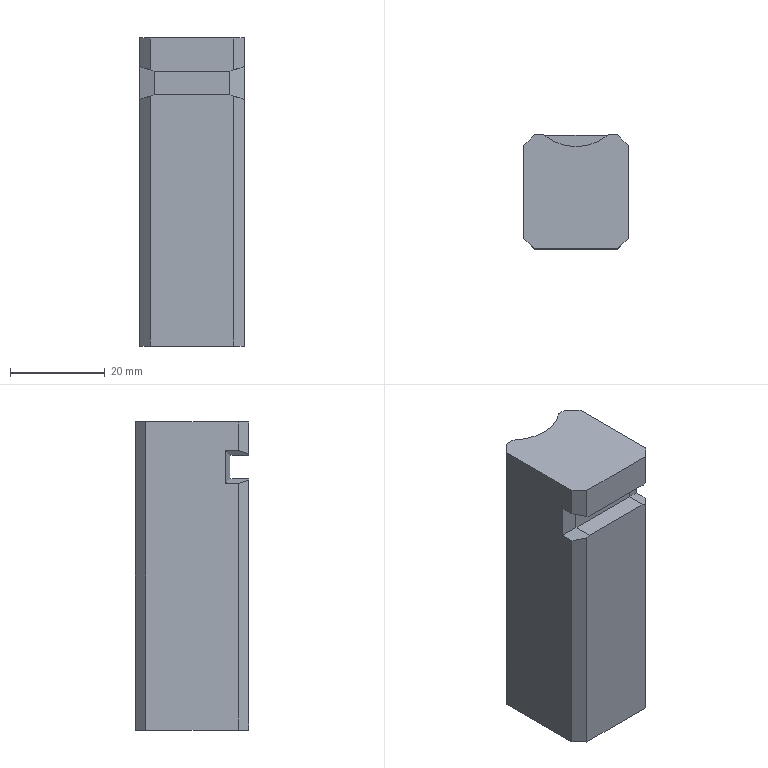Part | NX | features DIE-5 2 | 1 solid | 26 faces | box 22 x 24 x 65 mm | volume 30873 mm3 | plane 24 | cylinder 2 | commonest cylinder face diameters 18.003 x1 21 x1
STEP:
#1=CARTESIAN_POINT('',(2498.895,-772.622,823.716));
#2=VERTEX_POINT('',#1);
#3=CARTESIAN_POINT('',(2485.293,-772.622,823.716));
#4=VERTEX_POINT('',#3);
#5=CARTESIAN_POINT('',(2492.094,-764.622,823.716));
#6=DIRECTION('',(0.,0.,1.));
#7=DIRECTION('',(-1.,0.,0.));
#8=AXIS2_PLACEMENT_3D('',#5,#6,#7);
#9=CIRCLE('',#8,10.5);
#10=EDGE_CURVE('',#2,#4,#9,.F.);
#11=ORIENTED_EDGE('',*,*,#10,.F.);
#12=CARTESIAN_POINT('',(2500.894,-772.622,823.716));
#13=DIRECTION('',(1.,0.,0.));
#14=VECTOR('',#13,1000.);
#15=LINE('',#12,#14);
#16=EDGE_CURVE('',#4,#2,#15,.T.);
#17=ORIENTED_EDGE('',*,*,#16,.F.);
#18=EDGE_LOOP('',(#11,#17));
#19=FACE_BOUND('',#18,.T.);
#20=CARTESIAN_POINT('',(2325.094,-923.422,823.716));
#21=DIRECTION('',(0.,0.,-1.));
#22=DIRECTION('',(-1.,0.,0.));
#23=AXIS2_PLACEMENT_3D('',#20,#21,#22);
#24=PLANE('',#23);
#25=ADVANCED_FACE('',(#19),#24,.F.);
#26=CARTESIAN_POINT('',(2483.294,-772.622,805.716));
#27=VERTEX_POINT('',#26);
#28=CARTESIAN_POINT('',(2483.294,-772.622,870.716));
#29=VERTEX_POINT('',#28);
#30=CARTESIAN_POINT('',(2483.294,-772.622,776.516));
#31=DIRECTION('',(0.,0.,1.));
#32=VECTOR('',#31,1000.);
#33=LINE('',#30,#32);
#34=EDGE_CURVE('',#27,#29,#33,.T.);
#35=ORIENTED_EDGE('',*,*,#34,.T.);
#36=CARTESIAN_POINT('',(2485.293,-772.622,870.716));
#37=VERTEX_POINT('',#36);
#38=CARTESIAN_POINT('',(2492.094,-772.622,870.716));
#39=DIRECTION('',(-1.,0.,0.));
#40=VECTOR('',#39,1000.);
#41=LINE('',#38,#40);
#42=EDGE_CURVE('',#37,#29,#41,.T.);
#43=ORIENTED_EDGE('',*,*,#42,.F.);
#44=CARTESIAN_POINT('',(2485.293,-772.622,839.716));
#45=DIRECTION('',(0.,0.,-1.));
#46=VECTOR('',#45,1000.);
#47=LINE('',#44,#46);
#48=EDGE_CURVE('',#37,#4,#47,.T.);
#49=ORIENTED_EDGE('',*,*,#48,.T.);
#50=ORIENTED_EDGE('',*,*,#16,.T.);
#51=CARTESIAN_POINT('',(2498.895,-772.622,870.716));
#52=VERTEX_POINT('',#51);
#53=CARTESIAN_POINT('',(2498.895,-772.622,839.716));
#54=DIRECTION('',(0.,0.,1.));
#55=VECTOR('',#54,1000.);
#56=LINE('',#53,#55);
#57=EDGE_CURVE('',#2,#52,#56,.T.);
#58=ORIENTED_EDGE('',*,*,#57,.T.);
#59=CARTESIAN_POINT('',(2500.894,-772.622,870.716));
#60=VERTEX_POINT('',#59);
#61=CARTESIAN_POINT('',(2492.094,-772.622,870.716));
#62=DIRECTION('',(-1.,0.,0.));
#63=VECTOR('',#62,1000.);
#64=LINE('',#61,#63);
#65=EDGE_CURVE('',#60,#52,#64,.T.);
#66=ORIENTED_EDGE('',*,*,#65,.F.);
#67=CARTESIAN_POINT('',(2500.894,-772.622,805.716));
#68=VERTEX_POINT('',#67);
#69=CARTESIAN_POINT('',(2500.894,-772.622,776.516));
#70=DIRECTION('',(0.,0.,1.));
#71=VECTOR('',#70,1000.);
#72=LINE('',#69,#71);
#73=EDGE_CURVE('',#68,#60,#72,.T.);
#74=ORIENTED_EDGE('',*,*,#73,.F.);
#75=CARTESIAN_POINT('',(2500.894,-772.622,805.716));
#76=DIRECTION('',(-1.,0.,0.));
#77=VECTOR('',#76,1000.);
#78=LINE('',#75,#77);
#79=EDGE_CURVE('',#68,#27,#78,.T.);
#80=ORIENTED_EDGE('',*,*,#79,.T.);
#81=EDGE_LOOP('',(#35,#43,#49,#50,#58,#66,#74,#80));
#82=FACE_BOUND('',#81,.T.);
#83=CARTESIAN_POINT('',(2500.894,-772.622,776.516));
#84=DIRECTION('',(0.,1.,0.));
#85=DIRECTION('',(1.,0.,0.));
#86=AXIS2_PLACEMENT_3D('',#83,#84,#85);
#87=PLANE('',#86);
#88=ADVANCED_FACE('',(#82),#87,.T.);
#89=CARTESIAN_POINT('',(2483.092,-784.622,805.716));
#90=VERTEX_POINT('',#89);
#91=CARTESIAN_POINT('',(2492.094,-784.622,805.716));
#92=DIRECTION('',(0.,0.,-1.));
#93=DIRECTION('',(-1.,0.,0.));
#94=AXIS2_PLACEMENT_3D('',#91,#92,#93);
#95=CIRCLE('',#94,9.002);
#96=EDGE_CURVE('',#90,#90,#95,.T.);
#97=ORIENTED_EDGE('',*,*,#96,.F.);
#98=EDGE_LOOP('',(#97));
#99=FACE_BOUND('',#98,.T.);
#100=CARTESIAN_POINT('',(2483.294,-796.622,805.716));
#101=VERTEX_POINT('',#100);
#102=CARTESIAN_POINT('',(2500.894,-796.622,805.716));
#103=VERTEX_POINT('',#102);
#104=CARTESIAN_POINT('',(2483.294,-796.622,805.716));
#105=DIRECTION('',(1.,0.,0.));
#106=VECTOR('',#105,1000.);
#107=LINE('',#104,#106);
#108=EDGE_CURVE('',#101,#103,#107,.T.);
#109=ORIENTED_EDGE('',*,*,#108,.F.);
#110=CARTESIAN_POINT('',(2481.094,-794.422,805.716));
#111=VERTEX_POINT('',#110);
#112=CARTESIAN_POINT('',(1816.984,-130.312,805.716));
#113=DIRECTION('',(-0.7071,0.7071,0.));
#114=VECTOR('',#113,1000.);
#115=LINE('',#112,#114);
#116=EDGE_CURVE('',#101,#111,#115,.T.);
#117=ORIENTED_EDGE('',*,*,#116,.T.);
#118=CARTESIAN_POINT('',(2481.094,-774.822,805.716));
#119=VERTEX_POINT('',#118);
#120=CARTESIAN_POINT('',(2481.094,-854.137,805.716));
#121=DIRECTION('',(0.,1.,0.));
#122=VECTOR('',#121,1000.);
#123=LINE('',#120,#122);
#124=EDGE_CURVE('',#111,#119,#123,.T.);
#125=ORIENTED_EDGE('',*,*,#124,.T.);
#126=CARTESIAN_POINT('',(1745.969,-1509.947,805.716));
#127=DIRECTION('',(0.7071,0.7071,0.));
#128=VECTOR('',#127,1000.);
#129=LINE('',#126,#128);
#130=EDGE_CURVE('',#119,#27,#129,.T.);
#131=ORIENTED_EDGE('',*,*,#130,.T.);
#132=ORIENTED_EDGE('',*,*,#79,.F.);
#133=CARTESIAN_POINT('',(2503.094,-774.822,805.716));
#134=VERTEX_POINT('',#133);
#135=CARTESIAN_POINT('',(2503.094,-774.822,805.716));
#136=DIRECTION('',(-0.7071,0.7071,0.));
#137=VECTOR('',#136,1000.);
#138=LINE('',#135,#137);
#139=EDGE_CURVE('',#134,#68,#138,.T.);
#140=ORIENTED_EDGE('',*,*,#139,.F.);
#141=CARTESIAN_POINT('',(2503.094,-794.422,805.716));
#142=VERTEX_POINT('',#141);
#143=CARTESIAN_POINT('',(2503.094,-794.422,805.716));
#144=DIRECTION('',(0.,1.,0.));
#145=VECTOR('',#144,1000.);
#146=LINE('',#143,#145);
#147=EDGE_CURVE('',#142,#134,#146,.T.);
#148=ORIENTED_EDGE('',*,*,#147,.F.);
#149=CARTESIAN_POINT('',(2500.894,-796.622,805.716));
#150=DIRECTION('',(0.7071,0.7071,0.));
#151=VECTOR('',#150,1000.);
#152=LINE('',#149,#151);
#153=EDGE_CURVE('',#103,#142,#152,.T.);
#154=ORIENTED_EDGE('',*,*,#153,.F.);
#155=EDGE_LOOP('',(#109,#117,#125,#131,#132,#140,#148,#154));
#156=FACE_BOUND('',#155,.T.);
#157=CARTESIAN_POINT('',(1093.159,-854.137,805.716));
#158=DIRECTION('',(0.,0.,-1.));
#159=DIRECTION('',(1.,0.,0.));
#160=AXIS2_PLACEMENT_3D('',#157,#158,#159);
#161=PLANE('',#160);
#162=ADVANCED_FACE('',(#99,#156),#161,.T.);
#163=CARTESIAN_POINT('',(2500.894,-796.622,858.45));
#164=VERTEX_POINT('',#163);
#165=CARTESIAN_POINT('',(2500.894,-796.622,776.516));
#166=DIRECTION('',(0.,0.,1.));
#167=VECTOR('',#166,1000.);
#168=LINE('',#165,#167);
#169=EDGE_CURVE('',#103,#164,#168,.T.);
#170=ORIENTED_EDGE('',*,*,#169,.T.);
#171=CARTESIAN_POINT('',(2500.094,-796.622,858.716));
#172=VERTEX_POINT('',#171);
#173=CARTESIAN_POINT('',(2500.094,-796.622,858.716));
#174=DIRECTION('',(0.9487,0.,-0.3162));
#175=VECTOR('',#174,1000.);
#176=LINE('',#173,#175);
#177=EDGE_CURVE('',#172,#164,#176,.T.);
#178=ORIENTED_EDGE('',*,*,#177,.F.);
#179=CARTESIAN_POINT('',(2484.094,-796.622,858.716));
#180=VERTEX_POINT('',#179);
#181=CARTESIAN_POINT('',(2483.294,-796.622,858.716));
#182=DIRECTION('',(1.,0.,0.));
#183=VECTOR('',#182,1000.);
#184=LINE('',#181,#183);
#185=EDGE_CURVE('',#180,#172,#184,.T.);
#186=ORIENTED_EDGE('',*,*,#185,.F.);
#187=CARTESIAN_POINT('',(2483.294,-796.622,858.45));
#188=VERTEX_POINT('',#187);
#189=CARTESIAN_POINT('',(2458.714,-796.622,850.256));
#190=DIRECTION('',(-0.9487,0.,-0.3162));
#191=VECTOR('',#190,1000.);
#192=LINE('',#189,#191);
#193=EDGE_CURVE('',#180,#188,#192,.T.);
#194=ORIENTED_EDGE('',*,*,#193,.T.);
#195=CARTESIAN_POINT('',(2483.294,-796.622,776.516));
#196=DIRECTION('',(0.,0.,1.));
#197=VECTOR('',#196,1000.);
#198=LINE('',#195,#197);
#199=EDGE_CURVE('',#101,#188,#198,.T.);
#200=ORIENTED_EDGE('',*,*,#199,.F.);
#201=ORIENTED_EDGE('',*,*,#108,.T.);
#202=EDGE_LOOP('',(#170,#178,#186,#194,#200,#201));
#203=FACE_BOUND('',#202,.T.);
#204=CARTESIAN_POINT('',(2483.294,-796.622,776.516));
#205=DIRECTION('',(0.,-1.,0.));
#206=DIRECTION('',(-1.,0.,0.));
#207=AXIS2_PLACEMENT_3D('',#204,#205,#206);
#208=PLANE('',#207);
#209=ADVANCED_FACE('',(#203),#208,.T.);
#210=CARTESIAN_POINT('',(2503.094,-774.822,870.716));
#211=VERTEX_POINT('',#210);
#212=CARTESIAN_POINT('',(2503.094,-774.822,776.516));
#213=DIRECTION('',(0.,0.,1.));
#214=VECTOR('',#213,1000.);
#215=LINE('',#212,#214);
#216=EDGE_CURVE('',#134,#211,#215,.T.);
#217=ORIENTED_EDGE('',*,*,#216,.T.);
#218=CARTESIAN_POINT('',(2503.094,-794.422,870.716));
#219=VERTEX_POINT('',#218);
#220=CARTESIAN_POINT('',(2503.094,-781.122,870.716));
#221=DIRECTION('',(0.,1.,0.));
#222=VECTOR('',#221,1000.);
#223=LINE('',#220,#222);
#224=EDGE_CURVE('',#219,#211,#223,.T.);
#225=ORIENTED_EDGE('',*,*,#224,.F.);
#226=CARTESIAN_POINT('',(2503.094,-794.422,864.716));
#227=VERTEX_POINT('',#226);
#228=CARTESIAN_POINT('',(2503.094,-794.422,776.516));
#229=DIRECTION('',(0.,0.,1.));
#230=VECTOR('',#229,1000.);
#231=LINE('',#228,#230);
#232=EDGE_CURVE('',#227,#219,#231,.T.);
#233=ORIENTED_EDGE('',*,*,#232,.F.);
#234=CARTESIAN_POINT('',(2503.094,-791.622,864.716));
#235=VERTEX_POINT('',#234);
#236=CARTESIAN_POINT('',(2503.094,-794.422,864.716));
#237=DIRECTION('',(0.,-1.,0.));
#238=VECTOR('',#237,1000.);
#239=LINE('',#236,#238);
#240=EDGE_CURVE('',#235,#227,#239,.T.);
#241=ORIENTED_EDGE('',*,*,#240,.F.);
#242=CARTESIAN_POINT('',(2503.094,-791.622,857.716));
#243=VERTEX_POINT('',#242);
#244=CARTESIAN_POINT('',(2503.094,-791.622,873.516));
#245=DIRECTION('',(0.,0.,1.));
#246=VECTOR('',#245,1000.);
#247=LINE('',#244,#246);
#248=EDGE_CURVE('',#243,#235,#247,.T.);
#249=ORIENTED_EDGE('',*,*,#248,.F.);
#250=CARTESIAN_POINT('',(2503.094,-794.422,857.716));
#251=VERTEX_POINT('',#250);
#252=CARTESIAN_POINT('',(2503.094,-794.422,857.716));
#253=DIRECTION('',(0.,-1.,0.));
#254=VECTOR('',#253,1000.);
#255=LINE('',#252,#254);
#256=EDGE_CURVE('',#243,#251,#255,.T.);
#257=ORIENTED_EDGE('',*,*,#256,.T.);
#258=CARTESIAN_POINT('',(2503.094,-794.422,776.516));
#259=DIRECTION('',(0.,0.,1.));
#260=VECTOR('',#259,1000.);
#261=LINE('',#258,#260);
#262=EDGE_CURVE('',#142,#251,#261,.T.);
#263=ORIENTED_EDGE('',*,*,#262,.F.);
#264=ORIENTED_EDGE('',*,*,#147,.T.);
#265=EDGE_LOOP('',(#217,#225,#233,#241,#249,#257,#263,#264));
#266=FACE_BOUND('',#265,.T.);
#267=CARTESIAN_POINT('',(2503.094,-794.422,776.516));
#268=DIRECTION('',(1.,0.,0.));
#269=DIRECTION('',(0.,0.,-1.));
#270=AXIS2_PLACEMENT_3D('',#267,#268,#269);
#271=PLANE('',#270);
#272=ADVANCED_FACE('',(#266),#271,.T.);
#273=ORIENTED_EDGE('',*,*,#73,.T.);
#274=CARTESIAN_POINT('',(2502.244,-773.972,870.716));
#275=DIRECTION('',(-0.7071,0.7071,0.));
#276=VECTOR('',#275,1000.);
#277=LINE('',#274,#276);
#278=EDGE_CURVE('',#211,#60,#277,.T.);
#279=ORIENTED_EDGE('',*,*,#278,.F.);
#280=ORIENTED_EDGE('',*,*,#216,.F.);
#281=ORIENTED_EDGE('',*,*,#139,.T.);
#282=EDGE_LOOP('',(#273,#279,#280,#281));
#283=FACE_BOUND('',#282,.T.);
#284=CARTESIAN_POINT('',(2503.094,-774.822,776.516));
#285=DIRECTION('',(0.7071,0.7071,0.));
#286=DIRECTION('',(0.7071,-0.7071,0.));
#287=AXIS2_PLACEMENT_3D('',#284,#285,#286);
#288=PLANE('',#287);
#289=ADVANCED_FACE('',(#283),#288,.T.);
#290=ORIENTED_EDGE('',*,*,#262,.T.);
#291=CARTESIAN_POINT('',(2502.368,-795.148,857.958));
#292=DIRECTION('',(0.6882,0.6882,-0.2294));
#293=VECTOR('',#292,1000.);
#294=LINE('',#291,#293);
#295=EDGE_CURVE('',#164,#251,#294,.T.);
#296=ORIENTED_EDGE('',*,*,#295,.F.);
#297=ORIENTED_EDGE('',*,*,#169,.F.);
#298=ORIENTED_EDGE('',*,*,#153,.T.);
#299=EDGE_LOOP('',(#290,#296,#297,#298));
#300=FACE_BOUND('',#299,.T.);
#301=CARTESIAN_POINT('',(2500.894,-796.622,776.516));
#302=DIRECTION('',(0.7071,-0.7071,0.));
#303=DIRECTION('',(-0.7071,-0.7071,0.));
#304=AXIS2_PLACEMENT_3D('',#301,#302,#303);
#305=PLANE('',#304);
#306=ADVANCED_FACE('',(#300),#305,.T.);
#307=CARTESIAN_POINT('',(2481.094,-794.422,857.716));
#308=VERTEX_POINT('',#307);
#309=CARTESIAN_POINT('',(2481.094,-794.422,776.516));
#310=DIRECTION('',(0.,0.,1.));
#311=VECTOR('',#310,1000.);
#312=LINE('',#309,#311);
#313=EDGE_CURVE('',#111,#308,#312,.T.);
#314=ORIENTED_EDGE('',*,*,#313,.T.);
#315=CARTESIAN_POINT('',(2481.094,-791.622,857.716));
#316=VERTEX_POINT('',#315);
#317=CARTESIAN_POINT('',(2481.094,-794.422,857.716));
#318=DIRECTION('',(0.,-1.,0.));
#319=VECTOR('',#318,1000.);
#320=LINE('',#317,#319);
#321=EDGE_CURVE('',#316,#308,#320,.T.);
#322=ORIENTED_EDGE('',*,*,#321,.F.);
#323=CARTESIAN_POINT('',(2481.094,-791.622,864.716));
#324=VERTEX_POINT('',#323);
#325=CARTESIAN_POINT('',(2481.094,-791.622,873.516));
#326=DIRECTION('',(0.,0.,1.));
#327=VECTOR('',#326,1000.);
#328=LINE('',#325,#327);
#329=EDGE_CURVE('',#316,#324,#328,.T.);
#330=ORIENTED_EDGE('',*,*,#329,.T.);
#331=CARTESIAN_POINT('',(2481.094,-794.422,864.716));
#332=VERTEX_POINT('',#331);
#333=CARTESIAN_POINT('',(2481.094,-794.422,864.716));
#334=DIRECTION('',(0.,-1.,0.));
#335=VECTOR('',#334,1000.);
#336=LINE('',#333,#335);
#337=EDGE_CURVE('',#324,#332,#336,.T.);
#338=ORIENTED_EDGE('',*,*,#337,.T.);
#339=CARTESIAN_POINT('',(2481.094,-794.422,870.716));
#340=VERTEX_POINT('',#339);
#341=CARTESIAN_POINT('',(2481.094,-794.422,776.516));
#342=DIRECTION('',(0.,0.,1.));
#343=VECTOR('',#342,1000.);
#344=LINE('',#341,#343);
#345=EDGE_CURVE('',#332,#340,#344,.T.);
#346=ORIENTED_EDGE('',*,*,#345,.T.);
#347=CARTESIAN_POINT('',(2481.094,-774.822,870.716));
#348=VERTEX_POINT('',#347);
#349=CARTESIAN_POINT('',(2481.094,-794.422,870.716));
#350=DIRECTION('',(0.,1.,0.));
#351=VECTOR('',#350,1000.);
#352=LINE('',#349,#351);
#353=EDGE_CURVE('',#340,#348,#352,.T.);
#354=ORIENTED_EDGE('',*,*,#353,.T.);
#355=CARTESIAN_POINT('',(2481.094,-774.822,776.516));
#356=DIRECTION('',(0.,0.,1.));
#357=VECTOR('',#356,1000.);
#358=LINE('',#355,#357);
#359=EDGE_CURVE('',#119,#348,#358,.T.);
#360=ORIENTED_EDGE('',*,*,#359,.F.);
#361=ORIENTED_EDGE('',*,*,#124,.F.);
#362=EDGE_LOOP('',(#314,#322,#330,#338,#346,#354,#360,#361));
#363=FACE_BOUND('',#362,.T.);
#364=CARTESIAN_POINT('',(2481.094,-794.422,776.516));
#365=DIRECTION('',(-1.,0.,0.));
#366=DIRECTION('',(0.,0.,-1.));
#367=AXIS2_PLACEMENT_3D('',#364,#365,#366);
#368=PLANE('',#367);
#369=ADVANCED_FACE('',(#363),#368,.T.);
#370=ORIENTED_EDGE('',*,*,#359,.T.);
#371=CARTESIAN_POINT('',(2481.094,-774.822,870.716));
#372=DIRECTION('',(0.7071,0.7071,0.));
#373=VECTOR('',#372,1000.);
#374=LINE('',#371,#373);
#375=EDGE_CURVE('',#348,#29,#374,.T.);
#376=ORIENTED_EDGE('',*,*,#375,.T.);
#377=ORIENTED_EDGE('',*,*,#34,.F.);
#378=ORIENTED_EDGE('',*,*,#130,.F.);
#379=EDGE_LOOP('',(#370,#376,#377,#378));
#380=FACE_BOUND('',#379,.T.);
#381=CARTESIAN_POINT('',(2481.094,-774.822,776.516));
#382=DIRECTION('',(-0.7071,0.7071,0.));
#383=DIRECTION('',(-0.7071,-0.7071,0.));
#384=AXIS2_PLACEMENT_3D('',#381,#382,#383);
#385=PLANE('',#384);
#386=ADVANCED_FACE('',(#380),#385,.T.);
#387=ORIENTED_EDGE('',*,*,#199,.T.);
#388=CARTESIAN_POINT('',(2481.82,-795.148,857.958));
#389=DIRECTION('',(-0.6882,0.6882,-0.2294));
#390=VECTOR('',#389,1000.);
#391=LINE('',#388,#390);
#392=EDGE_CURVE('',#188,#308,#391,.T.);
#393=ORIENTED_EDGE('',*,*,#392,.T.);
#394=ORIENTED_EDGE('',*,*,#313,.F.);
#395=ORIENTED_EDGE('',*,*,#116,.F.);
#396=EDGE_LOOP('',(#387,#393,#394,#395));
#397=FACE_BOUND('',#396,.T.);
#398=CARTESIAN_POINT('',(2483.294,-796.622,776.516));
#399=DIRECTION('',(-0.7071,-0.7071,0.));
#400=DIRECTION('',(0.7071,-0.7071,0.));
#401=AXIS2_PLACEMENT_3D('',#398,#399,#400);
#402=PLANE('',#401);
#403=ADVANCED_FACE('',(#397),#402,.T.);
#404=CARTESIAN_POINT('',(2501.095,-784.622,810.716));
#405=VERTEX_POINT('',#404);
#406=CARTESIAN_POINT('',(2492.094,-784.622,810.716));
#407=DIRECTION('',(0.,0.,1.));
#408=DIRECTION('',(1.,0.,0.));
#409=AXIS2_PLACEMENT_3D('',#406,#407,#408);
#410=CIRCLE('',#409,9.002);
#411=EDGE_CURVE('',#405,#405,#410,.T.);
#412=ORIENTED_EDGE('',*,*,#411,.T.);
#413=EDGE_LOOP('',(#412));
#414=FACE_BOUND('',#413,.T.);
#415=ORIENTED_EDGE('',*,*,#96,.T.);
#416=EDGE_LOOP('',(#415));
#417=FACE_BOUND('',#416,.T.);
#418=CARTESIAN_POINT('',(2492.094,-784.622,790.516));
#419=DIRECTION('',(0.,0.,1.));
#420=DIRECTION('',(1.,0.,0.));
#421=AXIS2_PLACEMENT_3D('',#418,#419,#420);
#422=CYLINDRICAL_SURFACE('',#421,9.002);
#423=ADVANCED_FACE('',(#414,#417),#422,.F.);
#424=ORIENTED_EDGE('',*,*,#411,.F.);
#425=EDGE_LOOP('',(#424));
#426=FACE_BOUND('',#425,.T.);
#427=CARTESIAN_POINT('',(-816.547,-754.758,810.716));
#428=DIRECTION('',(0.,0.,1.));
#429=DIRECTION('',(1.,0.,0.));
#430=AXIS2_PLACEMENT_3D('',#427,#428,#429);
#431=PLANE('',#430);
#432=ADVANCED_FACE('',(#426),#431,.F.);
#433=CARTESIAN_POINT('',(2484.094,-792.622,863.716));
#434=VERTEX_POINT('',#433);
#435=CARTESIAN_POINT('',(2484.094,-796.622,863.716));
#436=VERTEX_POINT('',#435);
#437=CARTESIAN_POINT('',(2484.094,-781.122,863.716));
#438=DIRECTION('',(0.,-1.,0.));
#439=VECTOR('',#438,1000.);
#440=LINE('',#437,#439);
#441=EDGE_CURVE('',#434,#436,#440,.T.);
#442=ORIENTED_EDGE('',*,*,#441,.F.);
#443=CARTESIAN_POINT('',(2500.094,-792.622,863.716));
#444=VERTEX_POINT('',#443);
#445=CARTESIAN_POINT('',(2500.094,-792.622,863.716));
#446=DIRECTION('',(1.,0.,0.));
#447=VECTOR('',#446,1000.);
#448=LINE('',#445,#447);
#449=EDGE_CURVE('',#434,#444,#448,.T.);
#450=ORIENTED_EDGE('',*,*,#449,.T.);
#451=CARTESIAN_POINT('',(2500.094,-796.622,863.716));
#452=VERTEX_POINT('',#451);
#453=CARTESIAN_POINT('',(2500.094,-781.122,863.716));
#454=DIRECTION('',(0.,1.,0.));
#455=VECTOR('',#454,1000.);
#456=LINE('',#453,#455);
#457=EDGE_CURVE('',#452,#444,#456,.T.);
#458=ORIENTED_EDGE('',*,*,#457,.F.);
#459=CARTESIAN_POINT('',(2483.294,-796.622,863.716));
#460=DIRECTION('',(-1.,0.,0.));
#461=VECTOR('',#460,1000.);
#462=LINE('',#459,#461);
#463=EDGE_CURVE('',#452,#436,#462,.T.);
#464=ORIENTED_EDGE('',*,*,#463,.T.);
#465=EDGE_LOOP('',(#442,#450,#458,#464));
#466=FACE_BOUND('',#465,.T.);
#467=CARTESIAN_POINT('',(2492.094,-781.122,863.716));
#468=DIRECTION('',(0.,0.,1.));
#469=DIRECTION('',(1.,0.,0.));
#470=AXIS2_PLACEMENT_3D('',#467,#468,#469);
#471=PLANE('',#470);
#472=ADVANCED_FACE('',(#466),#471,.F.);
#473=ORIENTED_EDGE('',*,*,#449,.F.);
#474=CARTESIAN_POINT('',(2484.094,-792.622,858.716));
#475=VERTEX_POINT('',#474);
#476=CARTESIAN_POINT('',(2484.094,-792.622,873.516));
#477=DIRECTION('',(0.,0.,-1.));
#478=VECTOR('',#477,1000.);
#479=LINE('',#476,#478);
#480=EDGE_CURVE('',#434,#475,#479,.T.);
#481=ORIENTED_EDGE('',*,*,#480,.T.);
#482=CARTESIAN_POINT('',(2500.094,-792.622,858.716));
#483=VERTEX_POINT('',#482);
#484=CARTESIAN_POINT('',(2500.094,-792.622,858.716));
#485=DIRECTION('',(1.,0.,0.));
#486=VECTOR('',#485,1000.);
#487=LINE('',#484,#486);
#488=EDGE_CURVE('',#475,#483,#487,.T.);
#489=ORIENTED_EDGE('',*,*,#488,.T.);
#490=CARTESIAN_POINT('',(2500.094,-792.622,873.516));
#491=DIRECTION('',(0.,0.,-1.));
#492=VECTOR('',#491,1000.);
#493=LINE('',#490,#492);
#494=EDGE_CURVE('',#444,#483,#493,.T.);
#495=ORIENTED_EDGE('',*,*,#494,.F.);
#496=EDGE_LOOP('',(#473,#481,#489,#495));
#497=FACE_BOUND('',#496,.T.);
#498=CARTESIAN_POINT('',(2500.094,-792.622,873.516));
#499=DIRECTION('',(0.,-1.,0.));
#500=DIRECTION('',(0.,0.,-1.));
#501=AXIS2_PLACEMENT_3D('',#498,#499,#500);
#502=PLANE('',#501);
#503=ADVANCED_FACE('',(#497),#502,.T.);
#504=CARTESIAN_POINT('',(2483.294,-796.622,870.716));
#505=VERTEX_POINT('',#504);
#506=CARTESIAN_POINT('',(2500.894,-796.622,870.716));
#507=VERTEX_POINT('',#506);
#508=CARTESIAN_POINT('',(2492.094,-796.622,870.716));
#509=DIRECTION('',(1.,0.,0.));
#510=VECTOR('',#509,1000.);
#511=LINE('',#508,#510);
#512=EDGE_CURVE('',#505,#507,#511,.T.);
#513=ORIENTED_EDGE('',*,*,#512,.F.);
#514=CARTESIAN_POINT('',(2483.294,-796.622,863.983));
#515=VERTEX_POINT('',#514);
#516=CARTESIAN_POINT('',(2483.294,-796.622,776.516));
#517=DIRECTION('',(0.,0.,1.));
#518=VECTOR('',#517,1000.);
#519=LINE('',#516,#518);
#520=EDGE_CURVE('',#515,#505,#519,.T.);
#521=ORIENTED_EDGE('',*,*,#520,.F.);
#522=CARTESIAN_POINT('',(2525.374,-796.622,849.956));
#523=DIRECTION('',(0.9487,0.,-0.3162));
#524=VECTOR('',#523,1000.);
#525=LINE('',#522,#524);
#526=EDGE_CURVE('',#515,#436,#525,.T.);
#527=ORIENTED_EDGE('',*,*,#526,.T.);
#528=ORIENTED_EDGE('',*,*,#463,.F.);
#529=CARTESIAN_POINT('',(2500.894,-796.622,863.983));
#530=VERTEX_POINT('',#529);
#531=CARTESIAN_POINT('',(2458.814,-796.622,849.956));
#532=DIRECTION('',(-0.9487,0.,-0.3162));
#533=VECTOR('',#532,1000.);
#534=LINE('',#531,#533);
#535=EDGE_CURVE('',#530,#452,#534,.T.);
#536=ORIENTED_EDGE('',*,*,#535,.F.);
#537=CARTESIAN_POINT('',(2500.894,-796.622,776.516));
#538=DIRECTION('',(0.,0.,1.));
#539=VECTOR('',#538,1000.);
#540=LINE('',#537,#539);
#541=EDGE_CURVE('',#530,#507,#540,.T.);
#542=ORIENTED_EDGE('',*,*,#541,.T.);
#543=EDGE_LOOP('',(#513,#521,#527,#528,#536,#542));
#544=FACE_BOUND('',#543,.T.);
#545=CARTESIAN_POINT('',(2483.294,-796.622,776.516));
#546=DIRECTION('',(0.,-1.,0.));
#547=DIRECTION('',(-1.,0.,0.));
#548=AXIS2_PLACEMENT_3D('',#545,#546,#547);
#549=PLANE('',#548);
#550=ADVANCED_FACE('',(#544),#549,.T.);
#551=ORIENTED_EDGE('',*,*,#57,.F.);
#552=ORIENTED_EDGE('',*,*,#10,.T.);
#553=ORIENTED_EDGE('',*,*,#48,.F.);
#554=CARTESIAN_POINT('',(2492.094,-764.622,870.716));
#555=DIRECTION('',(0.,0.,-1.));
#556=DIRECTION('',(-1.,0.,0.));
#557=AXIS2_PLACEMENT_3D('',#554,#555,#556);
#558=CIRCLE('',#557,10.5);
#559=EDGE_CURVE('',#52,#37,#558,.T.);
#560=ORIENTED_EDGE('',*,*,#559,.F.);
#561=EDGE_LOOP('',(#551,#552,#553,#560));
#562=FACE_BOUND('',#561,.T.);
#563=CARTESIAN_POINT('',(2492.094,-764.622,858.716));
#564=DIRECTION('',(0.,0.,1.));
#565=DIRECTION('',(1.,0.,0.));
#566=AXIS2_PLACEMENT_3D('',#563,#564,#565);
#567=CYLINDRICAL_SURFACE('',#566,10.5);
#568=ADVANCED_FACE('',(#562),#567,.F.);
#569=ORIENTED_EDGE('',*,*,#488,.F.);
#570=CARTESIAN_POINT('',(2484.094,-781.122,858.716));
#571=DIRECTION('',(0.,-1.,0.));
#572=VECTOR('',#571,1000.);
#573=LINE('',#570,#572);
#574=EDGE_CURVE('',#475,#180,#573,.T.);
#575=ORIENTED_EDGE('',*,*,#574,.T.);
#576=ORIENTED_EDGE('',*,*,#185,.T.);
#577=CARTESIAN_POINT('',(2500.094,-781.122,858.716));
#578=DIRECTION('',(0.,-1.,0.));
#579=VECTOR('',#578,1000.);
#580=LINE('',#577,#579);
#581=EDGE_CURVE('',#483,#172,#580,.T.);
#582=ORIENTED_EDGE('',*,*,#581,.F.);
#583=EDGE_LOOP('',(#569,#575,#576,#582));
#584=FACE_BOUND('',#583,.T.);
#585=CARTESIAN_POINT('',(2492.094,-781.122,858.716));
#586=DIRECTION('',(0.,0.,1.));
#587=DIRECTION('',(1.,0.,0.));
#588=AXIS2_PLACEMENT_3D('',#585,#586,#587);
#589=PLANE('',#588);
#590=ADVANCED_FACE('',(#584),#589,.T.);
#591=CARTESIAN_POINT('',(2499.003,-792.986,863.353));
#592=DIRECTION('',(0.9045,0.3015,0.3015));
#593=VECTOR('',#592,1000.);
#594=LINE('',#591,#593);
#595=EDGE_CURVE('',#444,#235,#594,.T.);
#596=ORIENTED_EDGE('',*,*,#595,.F.);
#597=ORIENTED_EDGE('',*,*,#494,.T.);
#598=CARTESIAN_POINT('',(2499.276,-792.895,858.989));
#599=DIRECTION('',(-0.9045,-0.3015,0.3015));
#600=VECTOR('',#599,1000.);
#601=LINE('',#598,#600);
#602=EDGE_CURVE('',#243,#483,#601,.T.);
#603=ORIENTED_EDGE('',*,*,#602,.F.);
#604=ORIENTED_EDGE('',*,*,#248,.T.);
#605=EDGE_LOOP('',(#596,#597,#603,#604));
#606=FACE_BOUND('',#605,.T.);
#607=CARTESIAN_POINT('',(2503.094,-791.622,873.516));
#608=DIRECTION('',(0.3162,-0.9487,0.));
#609=DIRECTION('',(-0.9487,-0.3162,0.));
#610=AXIS2_PLACEMENT_3D('',#607,#608,#609);
#611=PLANE('',#610);
#612=ADVANCED_FACE('',(#606),#611,.T.);
#613=ORIENTED_EDGE('',*,*,#535,.T.);
#614=ORIENTED_EDGE('',*,*,#457,.T.);
#615=ORIENTED_EDGE('',*,*,#595,.T.);
#616=ORIENTED_EDGE('',*,*,#240,.T.);
#617=CARTESIAN_POINT('',(2500.473,-797.043,863.843));
#618=DIRECTION('',(0.6882,0.6882,0.2294));
#619=VECTOR('',#618,1000.);
#620=LINE('',#617,#619);
#621=EDGE_CURVE('',#530,#227,#620,.T.);
#622=ORIENTED_EDGE('',*,*,#621,.F.);
#623=EDGE_LOOP('',(#613,#614,#615,#616,#622));
#624=FACE_BOUND('',#623,.T.);
#625=CARTESIAN_POINT('',(2500.094,-796.622,863.716));
#626=DIRECTION('',(0.3162,0.,-0.9487));
#627=DIRECTION('',(-0.9487,0.,-0.3162));
#628=AXIS2_PLACEMENT_3D('',#625,#626,#627);
#629=PLANE('',#628);
#630=ADVANCED_FACE('',(#624),#629,.T.);
#631=ORIENTED_EDGE('',*,*,#621,.T.);
#632=ORIENTED_EDGE('',*,*,#232,.T.);
#633=CARTESIAN_POINT('',(2504.244,-793.272,870.716));
#634=DIRECTION('',(0.7071,0.7071,0.));
#635=VECTOR('',#634,1000.);
#636=LINE('',#633,#635);
#637=EDGE_CURVE('',#507,#219,#636,.T.);
#638=ORIENTED_EDGE('',*,*,#637,.F.);
#639=ORIENTED_EDGE('',*,*,#541,.F.);
#640=EDGE_LOOP('',(#631,#632,#638,#639));
#641=FACE_BOUND('',#640,.T.);
#642=CARTESIAN_POINT('',(2500.894,-796.622,776.516));
#643=DIRECTION('',(0.7071,-0.7071,0.));
#644=DIRECTION('',(-0.7071,-0.7071,0.));
#645=AXIS2_PLACEMENT_3D('',#642,#643,#644);
#646=PLANE('',#645);
#647=ADVANCED_FACE('',(#641),#646,.T.);
#648=ORIENTED_EDGE('',*,*,#581,.T.);
#649=ORIENTED_EDGE('',*,*,#177,.T.);
#650=ORIENTED_EDGE('',*,*,#295,.T.);
#651=ORIENTED_EDGE('',*,*,#256,.F.);
#652=ORIENTED_EDGE('',*,*,#602,.T.);
#653=EDGE_LOOP('',(#648,#649,#650,#651,#652));
#654=FACE_BOUND('',#653,.T.);
#655=CARTESIAN_POINT('',(2500.094,-792.622,858.716));
#656=DIRECTION('',(0.3162,0.,0.9487));
#657=DIRECTION('',(0.9487,0.,-0.3162));
#658=AXIS2_PLACEMENT_3D('',#655,#656,#657);
#659=PLANE('',#658);
#660=ADVANCED_FACE('',(#654),#659,.T.);
#661=CARTESIAN_POINT('',(2483.715,-797.043,863.843));
#662=DIRECTION('',(-0.6882,0.6882,0.2294));
#663=VECTOR('',#662,1000.);
#664=LINE('',#661,#663);
#665=EDGE_CURVE('',#515,#332,#664,.T.);
#666=ORIENTED_EDGE('',*,*,#665,.F.);
#667=ORIENTED_EDGE('',*,*,#520,.T.);
#668=CARTESIAN_POINT('',(2483.294,-796.622,870.716));
#669=DIRECTION('',(-0.7071,0.7071,0.));
#670=VECTOR('',#669,1000.);
#671=LINE('',#668,#670);
#672=EDGE_CURVE('',#505,#340,#671,.T.);
#673=ORIENTED_EDGE('',*,*,#672,.T.);
#674=ORIENTED_EDGE('',*,*,#345,.F.);
#675=EDGE_LOOP('',(#666,#667,#673,#674));
#676=FACE_BOUND('',#675,.T.);
#677=CARTESIAN_POINT('',(2483.294,-796.622,776.516));
#678=DIRECTION('',(-0.7071,-0.7071,0.));
#679=DIRECTION('',(0.7071,-0.7071,0.));
#680=AXIS2_PLACEMENT_3D('',#677,#678,#679);
#681=PLANE('',#680);
#682=ADVANCED_FACE('',(#676),#681,.T.);
#683=ORIENTED_EDGE('',*,*,#526,.F.);
#684=ORIENTED_EDGE('',*,*,#665,.T.);
#685=ORIENTED_EDGE('',*,*,#337,.F.);
#686=CARTESIAN_POINT('',(2485.185,-792.986,863.353));
#687=DIRECTION('',(-0.9045,0.3015,0.3015));
#688=VECTOR('',#687,1000.);
#689=LINE('',#686,#688);
#690=EDGE_CURVE('',#434,#324,#689,.T.);
#691=ORIENTED_EDGE('',*,*,#690,.F.);
#692=ORIENTED_EDGE('',*,*,#441,.T.);
#693=EDGE_LOOP('',(#683,#684,#685,#691,#692));
#694=FACE_BOUND('',#693,.T.);
#695=CARTESIAN_POINT('',(2484.094,-796.622,863.716));
#696=DIRECTION('',(-0.3162,0.,-0.9487));
#697=DIRECTION('',(0.9487,0.,-0.3162));
#698=AXIS2_PLACEMENT_3D('',#695,#696,#697);
#699=PLANE('',#698);
#700=ADVANCED_FACE('',(#694),#699,.T.);
#701=ORIENTED_EDGE('',*,*,#690,.T.);
#702=ORIENTED_EDGE('',*,*,#329,.F.);
#703=CARTESIAN_POINT('',(2484.912,-792.895,858.989));
#704=DIRECTION('',(0.9045,-0.3015,0.3015));
#705=VECTOR('',#704,1000.);
#706=LINE('',#703,#705);
#707=EDGE_CURVE('',#316,#475,#706,.T.);
#708=ORIENTED_EDGE('',*,*,#707,.T.);
#709=ORIENTED_EDGE('',*,*,#480,.F.);
#710=EDGE_LOOP('',(#701,#702,#708,#709));
#711=FACE_BOUND('',#710,.T.);
#712=CARTESIAN_POINT('',(2481.094,-791.622,873.516));
#713=DIRECTION('',(-0.3162,-0.9487,0.));
#714=DIRECTION('',(0.9487,-0.3162,0.));
#715=AXIS2_PLACEMENT_3D('',#712,#713,#714);
#716=PLANE('',#715);
#717=ADVANCED_FACE('',(#711),#716,.T.);
#718=ORIENTED_EDGE('',*,*,#65,.T.);
#719=ORIENTED_EDGE('',*,*,#559,.T.);
#720=ORIENTED_EDGE('',*,*,#42,.T.);
#721=ORIENTED_EDGE('',*,*,#375,.F.);
#722=ORIENTED_EDGE('',*,*,#353,.F.);
#723=ORIENTED_EDGE('',*,*,#672,.F.);
#724=ORIENTED_EDGE('',*,*,#512,.T.);
#725=ORIENTED_EDGE('',*,*,#637,.T.);
#726=ORIENTED_EDGE('',*,*,#224,.T.);
#727=ORIENTED_EDGE('',*,*,#278,.T.);
#728=EDGE_LOOP('',(#718,#719,#720,#721,#722,#723,#724,#725,#726,#727));
#729=FACE_BOUND('',#728,.T.);
#730=CARTESIAN_POINT('',(2492.094,-781.122,870.716));
#731=DIRECTION('',(0.,0.,1.));
#732=DIRECTION('',(1.,0.,0.));
#733=AXIS2_PLACEMENT_3D('',#730,#731,#732);
#734=PLANE('',#733);
#735=ADVANCED_FACE('',(#729),#734,.T.);
#736=ORIENTED_EDGE('',*,*,#574,.F.);
#737=ORIENTED_EDGE('',*,*,#707,.F.);
#738=ORIENTED_EDGE('',*,*,#321,.T.);
#739=ORIENTED_EDGE('',*,*,#392,.F.);
#740=ORIENTED_EDGE('',*,*,#193,.F.);
#741=EDGE_LOOP('',(#736,#737,#738,#739,#740));
#742=FACE_BOUND('',#741,.T.);
#743=CARTESIAN_POINT('',(2484.094,-792.622,858.716));
#744=DIRECTION('',(-0.3162,0.,0.9487));
#745=DIRECTION('',(-0.9487,0.,-0.3162));
#746=AXIS2_PLACEMENT_3D('',#743,#744,#745);
#747=PLANE('',#746);
#748=ADVANCED_FACE('',(#742),#747,.T.);
#749=CLOSED_SHELL('',(#25,#88,#162,#209,#272,#289,#306,#369,#386,#403,#423,#432,#472,#503,#550,#568,#590,#612,#630,#647,#660,#682,#700,#717,#735,#748));
#750=MANIFOLD_SOLID_BREP('',#749);
#751=(LENGTH_UNIT()NAMED_UNIT(*)SI_UNIT(.MILLI.,.METRE.));
#752=UNCERTAINTY_MEASURE_WITH_UNIT(LENGTH_MEASURE(0.00001),#751,'','');
#753=(NAMED_UNIT(*)PLANE_ANGLE_UNIT()SI_UNIT($,.RADIAN.));
#754=(NAMED_UNIT(*)SI_UNIT($,.STERADIAN.)SOLID_ANGLE_UNIT());
#755=(GEOMETRIC_REPRESENTATION_CONTEXT(3)GLOBAL_UNCERTAINTY_ASSIGNED_CONTEXT((#752))GLOBAL_UNIT_ASSIGNED_CONTEXT((#751,#753,#754))REPRESENTATION_CONTEXT('',''));
#756=ADVANCED_BREP_SHAPE_REPRESENTATION('',(#750),#755);